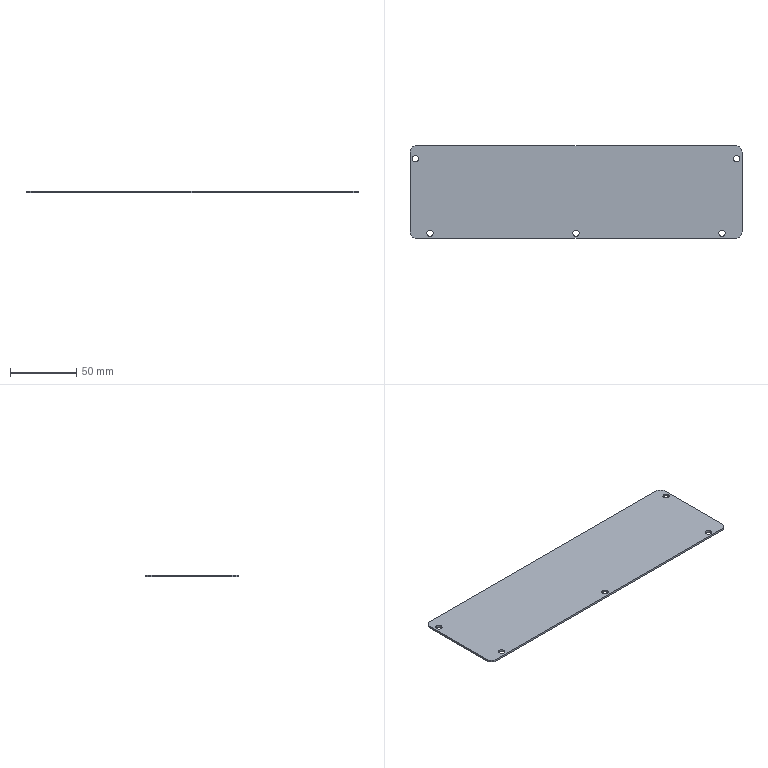Part | SolidWorks | features BreakCorner 1, FlatPattern 1, HoleWzd 1, SMBaseFlange 1, SheetMetal 1 | 1 solid | 20 faces | box 250 x 70 x 1.5 mm | volume 26082 mm3 | cylinder 14 | plane 6 | commonest cylinder face diameters 4.8 x10 10 x4
STEP:
#1=CARTESIAN_POINT('',(123.4,25.,0.));
#2=VERTEX_POINT('',#1);
#3=CARTESIAN_POINT('',(118.6,25.,0.));
#4=VERTEX_POINT('',#3);
#5=CARTESIAN_POINT('',(121.,25.,0.));
#6=DIRECTION('',(0.,0.,-1.));
#7=DIRECTION('',(-1.,0.,0.));
#8=AXIS2_PLACEMENT_3D('',#5,#6,#7);
#9=CIRCLE('',#8,2.4);
#10=EDGE_CURVE('',#2,#4,#9,.T.);
#11=ORIENTED_EDGE('',*,*,#10,.F.);
#12=CARTESIAN_POINT('',(123.4,25.,-1.5));
#13=VERTEX_POINT('',#12);
#14=CARTESIAN_POINT('',(123.4,25.,-1.5));
#15=DIRECTION('',(0.,0.,-1.));
#16=VECTOR('',#15,1000.);
#17=LINE('',#14,#16);
#18=EDGE_CURVE('',#2,#13,#17,.T.);
#19=ORIENTED_EDGE('',*,*,#18,.T.);
#20=CARTESIAN_POINT('',(118.6,25.,-1.5));
#21=VERTEX_POINT('',#20);
#22=CARTESIAN_POINT('',(121.,25.,-1.5));
#23=DIRECTION('',(0.,0.,-1.));
#24=DIRECTION('',(-1.,0.,0.));
#25=AXIS2_PLACEMENT_3D('',#22,#23,#24);
#26=CIRCLE('',#25,2.4);
#27=EDGE_CURVE('',#13,#21,#26,.T.);
#28=ORIENTED_EDGE('',*,*,#27,.T.);
#29=CARTESIAN_POINT('',(118.6,25.,-1.5));
#30=DIRECTION('',(0.,0.,-1.));
#31=VECTOR('',#30,1000.);
#32=LINE('',#29,#31);
#33=EDGE_CURVE('',#4,#21,#32,.T.);
#34=ORIENTED_EDGE('',*,*,#33,.F.);
#35=EDGE_LOOP('',(#11,#19,#28,#34));
#36=FACE_OUTER_BOUND('',#35,.T.);
#37=CARTESIAN_POINT('',(121.,25.,-1.5));
#38=DIRECTION('',(0.,0.,-1.));
#39=DIRECTION('',(-1.,0.,0.));
#40=AXIS2_PLACEMENT_3D('',#37,#38,#39);
#41=CYLINDRICAL_SURFACE('',#40,2.4);
#42=ADVANCED_FACE('',(#36),#41,.F.);
#43=CARTESIAN_POINT('',(112.4,-31.,0.));
#44=VERTEX_POINT('',#43);
#45=CARTESIAN_POINT('',(107.6,-31.,0.));
#46=VERTEX_POINT('',#45);
#47=CARTESIAN_POINT('',(110.,-31.,0.));
#48=DIRECTION('',(0.,0.,-1.));
#49=DIRECTION('',(-1.,0.,0.));
#50=AXIS2_PLACEMENT_3D('',#47,#48,#49);
#51=CIRCLE('',#50,2.4);
#52=EDGE_CURVE('',#44,#46,#51,.T.);
#53=ORIENTED_EDGE('',*,*,#52,.F.);
#54=CARTESIAN_POINT('',(112.4,-31.,-1.5));
#55=VERTEX_POINT('',#54);
#56=CARTESIAN_POINT('',(112.4,-31.,-1.5));
#57=DIRECTION('',(0.,0.,-1.));
#58=VECTOR('',#57,1000.);
#59=LINE('',#56,#58);
#60=EDGE_CURVE('',#44,#55,#59,.T.);
#61=ORIENTED_EDGE('',*,*,#60,.T.);
#62=CARTESIAN_POINT('',(107.6,-31.,-1.5));
#63=VERTEX_POINT('',#62);
#64=CARTESIAN_POINT('',(110.,-31.,-1.5));
#65=DIRECTION('',(0.,0.,-1.));
#66=DIRECTION('',(-1.,0.,0.));
#67=AXIS2_PLACEMENT_3D('',#64,#65,#66);
#68=CIRCLE('',#67,2.4);
#69=EDGE_CURVE('',#55,#63,#68,.T.);
#70=ORIENTED_EDGE('',*,*,#69,.T.);
#71=CARTESIAN_POINT('',(107.6,-31.,-1.5));
#72=DIRECTION('',(0.,0.,-1.));
#73=VECTOR('',#72,1000.);
#74=LINE('',#71,#73);
#75=EDGE_CURVE('',#46,#63,#74,.T.);
#76=ORIENTED_EDGE('',*,*,#75,.F.);
#77=EDGE_LOOP('',(#53,#61,#70,#76));
#78=FACE_OUTER_BOUND('',#77,.T.);
#79=CARTESIAN_POINT('',(110.,-31.,-1.5));
#80=DIRECTION('',(0.,0.,-1.));
#81=DIRECTION('',(-1.,0.,0.));
#82=AXIS2_PLACEMENT_3D('',#79,#80,#81);
#83=CYLINDRICAL_SURFACE('',#82,2.4);
#84=ADVANCED_FACE('',(#78),#83,.F.);
#85=CARTESIAN_POINT('',(2.4,-31.,0.));
#86=VERTEX_POINT('',#85);
#87=CARTESIAN_POINT('',(-2.4,-31.,0.));
#88=VERTEX_POINT('',#87);
#89=CARTESIAN_POINT('',(0.,-31.,0.));
#90=DIRECTION('',(0.,0.,-1.));
#91=DIRECTION('',(-1.,0.,0.));
#92=AXIS2_PLACEMENT_3D('',#89,#90,#91);
#93=CIRCLE('',#92,2.4);
#94=EDGE_CURVE('',#86,#88,#93,.T.);
#95=ORIENTED_EDGE('',*,*,#94,.F.);
#96=CARTESIAN_POINT('',(2.4,-31.,-1.5));
#97=VERTEX_POINT('',#96);
#98=CARTESIAN_POINT('',(2.4,-31.,-1.5));
#99=DIRECTION('',(0.,0.,-1.));
#100=VECTOR('',#99,1000.);
#101=LINE('',#98,#100);
#102=EDGE_CURVE('',#86,#97,#101,.T.);
#103=ORIENTED_EDGE('',*,*,#102,.T.);
#104=CARTESIAN_POINT('',(-2.4,-31.,-1.5));
#105=VERTEX_POINT('',#104);
#106=CARTESIAN_POINT('',(0.,-31.,-1.5));
#107=DIRECTION('',(0.,0.,-1.));
#108=DIRECTION('',(-1.,0.,0.));
#109=AXIS2_PLACEMENT_3D('',#106,#107,#108);
#110=CIRCLE('',#109,2.4);
#111=EDGE_CURVE('',#97,#105,#110,.T.);
#112=ORIENTED_EDGE('',*,*,#111,.T.);
#113=CARTESIAN_POINT('',(-2.4,-31.,-1.5));
#114=DIRECTION('',(0.,0.,-1.));
#115=VECTOR('',#114,1000.);
#116=LINE('',#113,#115);
#117=EDGE_CURVE('',#88,#105,#116,.T.);
#118=ORIENTED_EDGE('',*,*,#117,.F.);
#119=EDGE_LOOP('',(#95,#103,#112,#118));
#120=FACE_OUTER_BOUND('',#119,.T.);
#121=CARTESIAN_POINT('',(0.,-31.,-1.5));
#122=DIRECTION('',(0.,0.,-1.));
#123=DIRECTION('',(-1.,0.,0.));
#124=AXIS2_PLACEMENT_3D('',#121,#122,#123);
#125=CYLINDRICAL_SURFACE('',#124,2.4);
#126=ADVANCED_FACE('',(#120),#125,.F.);
#127=CARTESIAN_POINT('',(-107.6,-31.,0.));
#128=VERTEX_POINT('',#127);
#129=CARTESIAN_POINT('',(-112.4,-31.,0.));
#130=VERTEX_POINT('',#129);
#131=CARTESIAN_POINT('',(-110.,-31.,0.));
#132=DIRECTION('',(0.,0.,-1.));
#133=DIRECTION('',(-1.,0.,0.));
#134=AXIS2_PLACEMENT_3D('',#131,#132,#133);
#135=CIRCLE('',#134,2.4);
#136=EDGE_CURVE('',#128,#130,#135,.T.);
#137=ORIENTED_EDGE('',*,*,#136,.F.);
#138=CARTESIAN_POINT('',(-107.6,-31.,-1.5));
#139=VERTEX_POINT('',#138);
#140=CARTESIAN_POINT('',(-107.6,-31.,-1.5));
#141=DIRECTION('',(0.,0.,-1.));
#142=VECTOR('',#141,1000.);
#143=LINE('',#140,#142);
#144=EDGE_CURVE('',#128,#139,#143,.T.);
#145=ORIENTED_EDGE('',*,*,#144,.T.);
#146=CARTESIAN_POINT('',(-112.4,-31.,-1.5));
#147=VERTEX_POINT('',#146);
#148=CARTESIAN_POINT('',(-110.,-31.,-1.5));
#149=DIRECTION('',(0.,0.,-1.));
#150=DIRECTION('',(-1.,0.,0.));
#151=AXIS2_PLACEMENT_3D('',#148,#149,#150);
#152=CIRCLE('',#151,2.4);
#153=EDGE_CURVE('',#139,#147,#152,.T.);
#154=ORIENTED_EDGE('',*,*,#153,.T.);
#155=CARTESIAN_POINT('',(-112.4,-31.,-1.5));
#156=DIRECTION('',(0.,0.,-1.));
#157=VECTOR('',#156,1000.);
#158=LINE('',#155,#157);
#159=EDGE_CURVE('',#130,#147,#158,.T.);
#160=ORIENTED_EDGE('',*,*,#159,.F.);
#161=EDGE_LOOP('',(#137,#145,#154,#160));
#162=FACE_OUTER_BOUND('',#161,.T.);
#163=CARTESIAN_POINT('',(-110.,-31.,-1.5));
#164=DIRECTION('',(0.,0.,-1.));
#165=DIRECTION('',(-1.,0.,0.));
#166=AXIS2_PLACEMENT_3D('',#163,#164,#165);
#167=CYLINDRICAL_SURFACE('',#166,2.4);
#168=ADVANCED_FACE('',(#162),#167,.F.);
#169=CARTESIAN_POINT('',(-118.6,25.,0.));
#170=VERTEX_POINT('',#169);
#171=CARTESIAN_POINT('',(-123.4,25.,0.));
#172=VERTEX_POINT('',#171);
#173=CARTESIAN_POINT('',(-121.,25.,0.));
#174=DIRECTION('',(0.,0.,-1.));
#175=DIRECTION('',(-1.,0.,0.));
#176=AXIS2_PLACEMENT_3D('',#173,#174,#175);
#177=CIRCLE('',#176,2.4);
#178=EDGE_CURVE('',#170,#172,#177,.T.);
#179=ORIENTED_EDGE('',*,*,#178,.F.);
#180=CARTESIAN_POINT('',(-118.6,25.,-1.5));
#181=VERTEX_POINT('',#180);
#182=CARTESIAN_POINT('',(-118.6,25.,-1.5));
#183=DIRECTION('',(0.,0.,-1.));
#184=VECTOR('',#183,1000.);
#185=LINE('',#182,#184);
#186=EDGE_CURVE('',#170,#181,#185,.T.);
#187=ORIENTED_EDGE('',*,*,#186,.T.);
#188=CARTESIAN_POINT('',(-123.4,25.,-1.5));
#189=VERTEX_POINT('',#188);
#190=CARTESIAN_POINT('',(-121.,25.,-1.5));
#191=DIRECTION('',(0.,0.,-1.));
#192=DIRECTION('',(-1.,0.,0.));
#193=AXIS2_PLACEMENT_3D('',#190,#191,#192);
#194=CIRCLE('',#193,2.4);
#195=EDGE_CURVE('',#181,#189,#194,.T.);
#196=ORIENTED_EDGE('',*,*,#195,.T.);
#197=CARTESIAN_POINT('',(-123.4,25.,-1.5));
#198=DIRECTION('',(0.,0.,-1.));
#199=VECTOR('',#198,1000.);
#200=LINE('',#197,#199);
#201=EDGE_CURVE('',#172,#189,#200,.T.);
#202=ORIENTED_EDGE('',*,*,#201,.F.);
#203=EDGE_LOOP('',(#179,#187,#196,#202));
#204=FACE_OUTER_BOUND('',#203,.T.);
#205=CARTESIAN_POINT('',(-121.,25.,-1.5));
#206=DIRECTION('',(0.,0.,-1.));
#207=DIRECTION('',(-1.,0.,0.));
#208=AXIS2_PLACEMENT_3D('',#205,#206,#207);
#209=CYLINDRICAL_SURFACE('',#208,2.4);
#210=ADVANCED_FACE('',(#204),#209,.F.);
#211=CARTESIAN_POINT('',(125.,-30.,-1.5));
#212=VERTEX_POINT('',#211);
#213=CARTESIAN_POINT('',(125.,30.,-1.5));
#214=VERTEX_POINT('',#213);
#215=CARTESIAN_POINT('',(125.,-35.,-1.5));
#216=DIRECTION('',(0.,1.,0.));
#217=VECTOR('',#216,1000.);
#218=LINE('',#215,#217);
#219=EDGE_CURVE('',#212,#214,#218,.T.);
#220=ORIENTED_EDGE('',*,*,#219,.T.);
#221=CARTESIAN_POINT('',(125.,30.,0.));
#222=VERTEX_POINT('',#221);
#223=CARTESIAN_POINT('',(125.,30.,-1.5));
#224=DIRECTION('',(0.,0.,1.));
#225=VECTOR('',#224,1000.);
#226=LINE('',#223,#225);
#227=EDGE_CURVE('',#214,#222,#226,.T.);
#228=ORIENTED_EDGE('',*,*,#227,.T.);
#229=CARTESIAN_POINT('',(125.,-30.,0.));
#230=VERTEX_POINT('',#229);
#231=CARTESIAN_POINT('',(125.,-35.,0.));
#232=DIRECTION('',(0.,1.,0.));
#233=VECTOR('',#232,1000.);
#234=LINE('',#231,#233);
#235=EDGE_CURVE('',#230,#222,#234,.T.);
#236=ORIENTED_EDGE('',*,*,#235,.F.);
#237=CARTESIAN_POINT('',(125.,-30.,-1.5));
#238=DIRECTION('',(0.,0.,-1.));
#239=VECTOR('',#238,1000.);
#240=LINE('',#237,#239);
#241=EDGE_CURVE('',#230,#212,#240,.T.);
#242=ORIENTED_EDGE('',*,*,#241,.T.);
#243=EDGE_LOOP('',(#220,#228,#236,#242));
#244=FACE_OUTER_BOUND('',#243,.T.);
#245=CARTESIAN_POINT('',(125.,-35.,-1.5));
#246=DIRECTION('',(1.,0.,0.));
#247=DIRECTION('',(0.,0.,-1.));
#248=AXIS2_PLACEMENT_3D('',#245,#246,#247);
#249=PLANE('',#248);
#250=ADVANCED_FACE('',(#244),#249,.T.);
#251=CARTESIAN_POINT('',(-120.,-35.,0.));
#252=VERTEX_POINT('',#251);
#253=CARTESIAN_POINT('',(120.,-35.,0.));
#254=VERTEX_POINT('',#253);
#255=CARTESIAN_POINT('',(-125.,-35.,0.));
#256=DIRECTION('',(1.,0.,0.));
#257=VECTOR('',#256,1000.);
#258=LINE('',#255,#257);
#259=EDGE_CURVE('',#252,#254,#258,.T.);
#260=ORIENTED_EDGE('',*,*,#259,.F.);
#261=CARTESIAN_POINT('',(-120.,-35.,-1.5));
#262=VERTEX_POINT('',#261);
#263=CARTESIAN_POINT('',(-120.,-35.,-1.5));
#264=DIRECTION('',(0.,0.,-1.));
#265=VECTOR('',#264,1000.);
#266=LINE('',#263,#265);
#267=EDGE_CURVE('',#252,#262,#266,.T.);
#268=ORIENTED_EDGE('',*,*,#267,.T.);
#269=CARTESIAN_POINT('',(120.,-35.,-1.5));
#270=VERTEX_POINT('',#269);
#271=CARTESIAN_POINT('',(-125.,-35.,-1.5));
#272=DIRECTION('',(1.,0.,0.));
#273=VECTOR('',#272,1000.);
#274=LINE('',#271,#273);
#275=EDGE_CURVE('',#262,#270,#274,.T.);
#276=ORIENTED_EDGE('',*,*,#275,.T.);
#277=CARTESIAN_POINT('',(120.,-35.,-1.5));
#278=DIRECTION('',(0.,0.,1.));
#279=VECTOR('',#278,1000.);
#280=LINE('',#277,#279);
#281=EDGE_CURVE('',#270,#254,#280,.T.);
#282=ORIENTED_EDGE('',*,*,#281,.T.);
#283=EDGE_LOOP('',(#260,#268,#276,#282));
#284=FACE_OUTER_BOUND('',#283,.T.);
#285=CARTESIAN_POINT('',(-125.,-35.,-1.5));
#286=DIRECTION('',(0.,-1.,0.));
#287=DIRECTION('',(0.,0.,-1.));
#288=AXIS2_PLACEMENT_3D('',#285,#286,#287);
#289=PLANE('',#288);
#290=ADVANCED_FACE('',(#284),#289,.T.);
#291=CARTESIAN_POINT('',(-125.,30.,0.));
#292=VERTEX_POINT('',#291);
#293=CARTESIAN_POINT('',(-125.,-30.,0.));
#294=VERTEX_POINT('',#293);
#295=CARTESIAN_POINT('',(-125.,-35.,0.));
#296=DIRECTION('',(0.,-1.,0.));
#297=VECTOR('',#296,1000.);
#298=LINE('',#295,#297);
#299=EDGE_CURVE('',#292,#294,#298,.T.);
#300=ORIENTED_EDGE('',*,*,#299,.F.);
#301=CARTESIAN_POINT('',(-125.,30.,-1.5));
#302=VERTEX_POINT('',#301);
#303=CARTESIAN_POINT('',(-125.,30.,-1.5));
#304=DIRECTION('',(0.,0.,-1.));
#305=VECTOR('',#304,1000.);
#306=LINE('',#303,#305);
#307=EDGE_CURVE('',#292,#302,#306,.T.);
#308=ORIENTED_EDGE('',*,*,#307,.T.);
#309=CARTESIAN_POINT('',(-125.,-30.,-1.5));
#310=VERTEX_POINT('',#309);
#311=CARTESIAN_POINT('',(-125.,-35.,-1.5));
#312=DIRECTION('',(0.,-1.,0.));
#313=VECTOR('',#312,1000.);
#314=LINE('',#311,#313);
#315=EDGE_CURVE('',#302,#310,#314,.T.);
#316=ORIENTED_EDGE('',*,*,#315,.T.);
#317=CARTESIAN_POINT('',(-125.,-30.,-1.5));
#318=DIRECTION('',(0.,0.,1.));
#319=VECTOR('',#318,1000.);
#320=LINE('',#317,#319);
#321=EDGE_CURVE('',#310,#294,#320,.T.);
#322=ORIENTED_EDGE('',*,*,#321,.T.);
#323=EDGE_LOOP('',(#300,#308,#316,#322));
#324=FACE_OUTER_BOUND('',#323,.T.);
#325=CARTESIAN_POINT('',(-125.,-35.,-1.5));
#326=DIRECTION('',(-1.,0.,0.));
#327=DIRECTION('',(0.,0.,1.));
#328=AXIS2_PLACEMENT_3D('',#325,#326,#327);
#329=PLANE('',#328);
#330=ADVANCED_FACE('',(#324),#329,.T.);
#331=CARTESIAN_POINT('',(120.,35.,0.));
#332=VERTEX_POINT('',#331);
#333=CARTESIAN_POINT('',(-120.,35.,0.));
#334=VERTEX_POINT('',#333);
#335=CARTESIAN_POINT('',(-125.,35.,0.));
#336=DIRECTION('',(-1.,0.,0.));
#337=VECTOR('',#336,1000.);
#338=LINE('',#335,#337);
#339=EDGE_CURVE('',#332,#334,#338,.T.);
#340=ORIENTED_EDGE('',*,*,#339,.F.);
#341=CARTESIAN_POINT('',(120.,35.,-1.5));
#342=VERTEX_POINT('',#341);
#343=CARTESIAN_POINT('',(120.,35.,-1.5));
#344=DIRECTION('',(0.,0.,-1.));
#345=VECTOR('',#344,1000.);
#346=LINE('',#343,#345);
#347=EDGE_CURVE('',#332,#342,#346,.T.);
#348=ORIENTED_EDGE('',*,*,#347,.T.);
#349=CARTESIAN_POINT('',(-120.,35.,-1.5));
#350=VERTEX_POINT('',#349);
#351=CARTESIAN_POINT('',(-125.,35.,-1.5));
#352=DIRECTION('',(-1.,0.,0.));
#353=VECTOR('',#352,1000.);
#354=LINE('',#351,#353);
#355=EDGE_CURVE('',#342,#350,#354,.T.);
#356=ORIENTED_EDGE('',*,*,#355,.T.);
#357=CARTESIAN_POINT('',(-120.,35.,-1.5));
#358=DIRECTION('',(0.,0.,1.));
#359=VECTOR('',#358,1000.);
#360=LINE('',#357,#359);
#361=EDGE_CURVE('',#350,#334,#360,.T.);
#362=ORIENTED_EDGE('',*,*,#361,.T.);
#363=EDGE_LOOP('',(#340,#348,#356,#362));
#364=FACE_OUTER_BOUND('',#363,.T.);
#365=CARTESIAN_POINT('',(-125.,35.,-1.5));
#366=DIRECTION('',(0.,1.,0.));
#367=DIRECTION('',(0.,0.,1.));
#368=AXIS2_PLACEMENT_3D('',#365,#366,#367);
#369=PLANE('',#368);
#370=ADVANCED_FACE('',(#364),#369,.T.);
#371=CARTESIAN_POINT('',(121.,25.,-1.5));
#372=DIRECTION('',(0.,0.,-1.));
#373=DIRECTION('',(-1.,0.,0.));
#374=AXIS2_PLACEMENT_3D('',#371,#372,#373);
#375=CIRCLE('',#374,2.4);
#376=EDGE_CURVE('',#21,#13,#375,.T.);
#377=ORIENTED_EDGE('',*,*,#376,.F.);
#378=ORIENTED_EDGE('',*,*,#27,.F.);
#379=EDGE_LOOP('',(#377,#378));
#380=FACE_BOUND('',#379,.T.);
#381=CARTESIAN_POINT('',(110.,-31.,-1.5));
#382=DIRECTION('',(0.,0.,-1.));
#383=DIRECTION('',(-1.,0.,0.));
#384=AXIS2_PLACEMENT_3D('',#381,#382,#383);
#385=CIRCLE('',#384,2.4);
#386=EDGE_CURVE('',#63,#55,#385,.T.);
#387=ORIENTED_EDGE('',*,*,#386,.F.);
#388=ORIENTED_EDGE('',*,*,#69,.F.);
#389=EDGE_LOOP('',(#387,#388));
#390=FACE_BOUND('',#389,.T.);
#391=CARTESIAN_POINT('',(0.,-31.,-1.5));
#392=DIRECTION('',(0.,0.,-1.));
#393=DIRECTION('',(-1.,0.,0.));
#394=AXIS2_PLACEMENT_3D('',#391,#392,#393);
#395=CIRCLE('',#394,2.4);
#396=EDGE_CURVE('',#105,#97,#395,.T.);
#397=ORIENTED_EDGE('',*,*,#396,.F.);
#398=ORIENTED_EDGE('',*,*,#111,.F.);
#399=EDGE_LOOP('',(#397,#398));
#400=FACE_BOUND('',#399,.T.);
#401=CARTESIAN_POINT('',(-110.,-31.,-1.5));
#402=DIRECTION('',(0.,0.,-1.));
#403=DIRECTION('',(-1.,0.,0.));
#404=AXIS2_PLACEMENT_3D('',#401,#402,#403);
#405=CIRCLE('',#404,2.4);
#406=EDGE_CURVE('',#147,#139,#405,.T.);
#407=ORIENTED_EDGE('',*,*,#406,.F.);
#408=ORIENTED_EDGE('',*,*,#153,.F.);
#409=EDGE_LOOP('',(#407,#408));
#410=FACE_BOUND('',#409,.T.);
#411=CARTESIAN_POINT('',(-121.,25.,-1.5));
#412=DIRECTION('',(0.,0.,-1.));
#413=DIRECTION('',(-1.,0.,0.));
#414=AXIS2_PLACEMENT_3D('',#411,#412,#413);
#415=CIRCLE('',#414,2.4);
#416=EDGE_CURVE('',#189,#181,#415,.T.);
#417=ORIENTED_EDGE('',*,*,#416,.F.);
#418=ORIENTED_EDGE('',*,*,#195,.F.);
#419=EDGE_LOOP('',(#417,#418));
#420=FACE_BOUND('',#419,.T.);
#421=ORIENTED_EDGE('',*,*,#355,.F.);
#422=CARTESIAN_POINT('',(120.,30.,-1.5));
#423=DIRECTION('',(0.,0.,-1.));
#424=DIRECTION('',(-1.,0.,0.));
#425=AXIS2_PLACEMENT_3D('',#422,#423,#424);
#426=CIRCLE('',#425,5.);
#427=EDGE_CURVE('',#342,#214,#426,.T.);
#428=ORIENTED_EDGE('',*,*,#427,.T.);
#429=ORIENTED_EDGE('',*,*,#219,.F.);
#430=CARTESIAN_POINT('',(120.,-30.,-1.5));
#431=DIRECTION('',(0.,0.,-1.));
#432=DIRECTION('',(-1.,0.,0.));
#433=AXIS2_PLACEMENT_3D('',#430,#431,#432);
#434=CIRCLE('',#433,5.);
#435=EDGE_CURVE('',#212,#270,#434,.T.);
#436=ORIENTED_EDGE('',*,*,#435,.T.);
#437=ORIENTED_EDGE('',*,*,#275,.F.);
#438=CARTESIAN_POINT('',(-120.,-30.,-1.5));
#439=DIRECTION('',(0.,0.,-1.));
#440=DIRECTION('',(-1.,0.,0.));
#441=AXIS2_PLACEMENT_3D('',#438,#439,#440);
#442=CIRCLE('',#441,5.);
#443=EDGE_CURVE('',#262,#310,#442,.T.);
#444=ORIENTED_EDGE('',*,*,#443,.T.);
#445=ORIENTED_EDGE('',*,*,#315,.F.);
#446=CARTESIAN_POINT('',(-120.,30.,-1.5));
#447=DIRECTION('',(0.,0.,-1.));
#448=DIRECTION('',(-1.,0.,0.));
#449=AXIS2_PLACEMENT_3D('',#446,#447,#448);
#450=CIRCLE('',#449,5.);
#451=EDGE_CURVE('',#302,#350,#450,.T.);
#452=ORIENTED_EDGE('',*,*,#451,.T.);
#453=EDGE_LOOP('',(#421,#428,#429,#436,#437,#444,#445,#452));
#454=FACE_OUTER_BOUND('',#453,.T.);
#455=CARTESIAN_POINT('',(0.,0.,-1.5));
#456=DIRECTION('',(0.,0.,-1.));
#457=DIRECTION('',(-1.,0.,0.));
#458=AXIS2_PLACEMENT_3D('',#455,#456,#457);
#459=PLANE('',#458);
#460=ADVANCED_FACE('',(#380,#390,#400,#410,#420,#454),#459,.T.);
#461=CARTESIAN_POINT('',(121.,25.,0.));
#462=DIRECTION('',(0.,0.,-1.));
#463=DIRECTION('',(-1.,0.,0.));
#464=AXIS2_PLACEMENT_3D('',#461,#462,#463);
#465=CIRCLE('',#464,2.4);
#466=EDGE_CURVE('',#4,#2,#465,.T.);
#467=ORIENTED_EDGE('',*,*,#466,.T.);
#468=ORIENTED_EDGE('',*,*,#10,.T.);
#469=EDGE_LOOP('',(#467,#468));
#470=FACE_BOUND('',#469,.T.);
#471=CARTESIAN_POINT('',(110.,-31.,0.));
#472=DIRECTION('',(0.,0.,-1.));
#473=DIRECTION('',(-1.,0.,0.));
#474=AXIS2_PLACEMENT_3D('',#471,#472,#473);
#475=CIRCLE('',#474,2.4);
#476=EDGE_CURVE('',#46,#44,#475,.T.);
#477=ORIENTED_EDGE('',*,*,#476,.T.);
#478=ORIENTED_EDGE('',*,*,#52,.T.);
#479=EDGE_LOOP('',(#477,#478));
#480=FACE_BOUND('',#479,.T.);
#481=CARTESIAN_POINT('',(0.,-31.,0.));
#482=DIRECTION('',(0.,0.,-1.));
#483=DIRECTION('',(-1.,0.,0.));
#484=AXIS2_PLACEMENT_3D('',#481,#482,#483);
#485=CIRCLE('',#484,2.4);
#486=EDGE_CURVE('',#88,#86,#485,.T.);
#487=ORIENTED_EDGE('',*,*,#486,.T.);
#488=ORIENTED_EDGE('',*,*,#94,.T.);
#489=EDGE_LOOP('',(#487,#488));
#490=FACE_BOUND('',#489,.T.);
#491=CARTESIAN_POINT('',(-110.,-31.,0.));
#492=DIRECTION('',(0.,0.,-1.));
#493=DIRECTION('',(-1.,0.,0.));
#494=AXIS2_PLACEMENT_3D('',#491,#492,#493);
#495=CIRCLE('',#494,2.4);
#496=EDGE_CURVE('',#130,#128,#495,.T.);
#497=ORIENTED_EDGE('',*,*,#496,.T.);
#498=ORIENTED_EDGE('',*,*,#136,.T.);
#499=EDGE_LOOP('',(#497,#498));
#500=FACE_BOUND('',#499,.T.);
#501=CARTESIAN_POINT('',(-121.,25.,0.));
#502=DIRECTION('',(0.,0.,-1.));
#503=DIRECTION('',(-1.,0.,0.));
#504=AXIS2_PLACEMENT_3D('',#501,#502,#503);
#505=CIRCLE('',#504,2.4);
#506=EDGE_CURVE('',#172,#170,#505,.T.);
#507=ORIENTED_EDGE('',*,*,#506,.T.);
#508=ORIENTED_EDGE('',*,*,#178,.T.);
#509=EDGE_LOOP('',(#507,#508));
#510=FACE_BOUND('',#509,.T.);
#511=ORIENTED_EDGE('',*,*,#235,.T.);
#512=CARTESIAN_POINT('',(120.,30.,0.));
#513=DIRECTION('',(0.,0.,1.));
#514=DIRECTION('',(-1.,0.,0.));
#515=AXIS2_PLACEMENT_3D('',#512,#513,#514);
#516=CIRCLE('',#515,5.);
#517=EDGE_CURVE('',#222,#332,#516,.T.);
#518=ORIENTED_EDGE('',*,*,#517,.T.);
#519=ORIENTED_EDGE('',*,*,#339,.T.);
#520=CARTESIAN_POINT('',(-120.,30.,0.));
#521=DIRECTION('',(0.,0.,1.));
#522=DIRECTION('',(-1.,0.,0.));
#523=AXIS2_PLACEMENT_3D('',#520,#521,#522);
#524=CIRCLE('',#523,5.);
#525=EDGE_CURVE('',#334,#292,#524,.T.);
#526=ORIENTED_EDGE('',*,*,#525,.T.);
#527=ORIENTED_EDGE('',*,*,#299,.T.);
#528=CARTESIAN_POINT('',(-120.,-30.,0.));
#529=DIRECTION('',(0.,0.,1.));
#530=DIRECTION('',(-1.,0.,0.));
#531=AXIS2_PLACEMENT_3D('',#528,#529,#530);
#532=CIRCLE('',#531,5.);
#533=EDGE_CURVE('',#294,#252,#532,.T.);
#534=ORIENTED_EDGE('',*,*,#533,.T.);
#535=ORIENTED_EDGE('',*,*,#259,.T.);
#536=CARTESIAN_POINT('',(120.,-30.,0.));
#537=DIRECTION('',(0.,0.,1.));
#538=DIRECTION('',(-1.,0.,0.));
#539=AXIS2_PLACEMENT_3D('',#536,#537,#538);
#540=CIRCLE('',#539,5.);
#541=EDGE_CURVE('',#254,#230,#540,.T.);
#542=ORIENTED_EDGE('',*,*,#541,.T.);
#543=EDGE_LOOP('',(#511,#518,#519,#526,#527,#534,#535,#542));
#544=FACE_OUTER_BOUND('',#543,.T.);
#545=CARTESIAN_POINT('',(0.,0.,0.));
#546=DIRECTION('',(0.,0.,-1.));
#547=DIRECTION('',(-1.,0.,0.));
#548=AXIS2_PLACEMENT_3D('',#545,#546,#547);
#549=PLANE('',#548);
#550=ADVANCED_FACE('',(#470,#480,#490,#500,#510,#544),#549,.F.);
#551=ORIENTED_EDGE('',*,*,#186,.F.);
#552=ORIENTED_EDGE('',*,*,#506,.F.);
#553=ORIENTED_EDGE('',*,*,#201,.T.);
#554=ORIENTED_EDGE('',*,*,#416,.T.);
#555=EDGE_LOOP('',(#551,#552,#553,#554));
#556=FACE_OUTER_BOUND('',#555,.T.);
#557=CARTESIAN_POINT('',(-121.,25.,-1.5));
#558=DIRECTION('',(0.,0.,-1.));
#559=DIRECTION('',(-1.,0.,0.));
#560=AXIS2_PLACEMENT_3D('',#557,#558,#559);
#561=CYLINDRICAL_SURFACE('',#560,2.4);
#562=ADVANCED_FACE('',(#556),#561,.F.);
#563=ORIENTED_EDGE('',*,*,#144,.F.);
#564=ORIENTED_EDGE('',*,*,#496,.F.);
#565=ORIENTED_EDGE('',*,*,#159,.T.);
#566=ORIENTED_EDGE('',*,*,#406,.T.);
#567=EDGE_LOOP('',(#563,#564,#565,#566));
#568=FACE_OUTER_BOUND('',#567,.T.);
#569=CARTESIAN_POINT('',(-110.,-31.,-1.5));
#570=DIRECTION('',(0.,0.,-1.));
#571=DIRECTION('',(-1.,0.,0.));
#572=AXIS2_PLACEMENT_3D('',#569,#570,#571);
#573=CYLINDRICAL_SURFACE('',#572,2.4);
#574=ADVANCED_FACE('',(#568),#573,.F.);
#575=ORIENTED_EDGE('',*,*,#102,.F.);
#576=ORIENTED_EDGE('',*,*,#486,.F.);
#577=ORIENTED_EDGE('',*,*,#117,.T.);
#578=ORIENTED_EDGE('',*,*,#396,.T.);
#579=EDGE_LOOP('',(#575,#576,#577,#578));
#580=FACE_OUTER_BOUND('',#579,.T.);
#581=CARTESIAN_POINT('',(0.,-31.,-1.5));
#582=DIRECTION('',(0.,0.,-1.));
#583=DIRECTION('',(-1.,0.,0.));
#584=AXIS2_PLACEMENT_3D('',#581,#582,#583);
#585=CYLINDRICAL_SURFACE('',#584,2.4);
#586=ADVANCED_FACE('',(#580),#585,.F.);
#587=ORIENTED_EDGE('',*,*,#60,.F.);
#588=ORIENTED_EDGE('',*,*,#476,.F.);
#589=ORIENTED_EDGE('',*,*,#75,.T.);
#590=ORIENTED_EDGE('',*,*,#386,.T.);
#591=EDGE_LOOP('',(#587,#588,#589,#590));
#592=FACE_OUTER_BOUND('',#591,.T.);
#593=CARTESIAN_POINT('',(110.,-31.,-1.5));
#594=DIRECTION('',(0.,0.,-1.));
#595=DIRECTION('',(-1.,0.,0.));
#596=AXIS2_PLACEMENT_3D('',#593,#594,#595);
#597=CYLINDRICAL_SURFACE('',#596,2.4);
#598=ADVANCED_FACE('',(#592),#597,.F.);
#599=ORIENTED_EDGE('',*,*,#18,.F.);
#600=ORIENTED_EDGE('',*,*,#466,.F.);
#601=ORIENTED_EDGE('',*,*,#33,.T.);
#602=ORIENTED_EDGE('',*,*,#376,.T.);
#603=EDGE_LOOP('',(#599,#600,#601,#602));
#604=FACE_OUTER_BOUND('',#603,.T.);
#605=CARTESIAN_POINT('',(121.,25.,-1.5));
#606=DIRECTION('',(0.,0.,-1.));
#607=DIRECTION('',(-1.,0.,0.));
#608=AXIS2_PLACEMENT_3D('',#605,#606,#607);
#609=CYLINDRICAL_SURFACE('',#608,2.4);
#610=ADVANCED_FACE('',(#604),#609,.F.);
#611=ORIENTED_EDGE('',*,*,#427,.F.);
#612=ORIENTED_EDGE('',*,*,#347,.F.);
#613=ORIENTED_EDGE('',*,*,#517,.F.);
#614=ORIENTED_EDGE('',*,*,#227,.F.);
#615=EDGE_LOOP('',(#611,#612,#613,#614));
#616=FACE_OUTER_BOUND('',#615,.T.);
#617=CARTESIAN_POINT('',(120.,30.,-1.5));
#618=DIRECTION('',(0.,0.,1.));
#619=DIRECTION('',(1.,0.,0.));
#620=AXIS2_PLACEMENT_3D('',#617,#618,#619);
#621=CYLINDRICAL_SURFACE('',#620,5.);
#622=ADVANCED_FACE('',(#616),#621,.T.);
#623=ORIENTED_EDGE('',*,*,#451,.F.);
#624=ORIENTED_EDGE('',*,*,#307,.F.);
#625=ORIENTED_EDGE('',*,*,#525,.F.);
#626=ORIENTED_EDGE('',*,*,#361,.F.);
#627=EDGE_LOOP('',(#623,#624,#625,#626));
#628=FACE_OUTER_BOUND('',#627,.T.);
#629=CARTESIAN_POINT('',(-120.,30.,-1.5));
#630=DIRECTION('',(0.,0.,1.));
#631=DIRECTION('',(1.,0.,0.));
#632=AXIS2_PLACEMENT_3D('',#629,#630,#631);
#633=CYLINDRICAL_SURFACE('',#632,5.);
#634=ADVANCED_FACE('',(#628),#633,.T.);
#635=ORIENTED_EDGE('',*,*,#443,.F.);
#636=ORIENTED_EDGE('',*,*,#267,.F.);
#637=ORIENTED_EDGE('',*,*,#533,.F.);
#638=ORIENTED_EDGE('',*,*,#321,.F.);
#639=EDGE_LOOP('',(#635,#636,#637,#638));
#640=FACE_OUTER_BOUND('',#639,.T.);
#641=CARTESIAN_POINT('',(-120.,-30.,-1.5));
#642=DIRECTION('',(0.,0.,1.));
#643=DIRECTION('',(1.,0.,0.));
#644=AXIS2_PLACEMENT_3D('',#641,#642,#643);
#645=CYLINDRICAL_SURFACE('',#644,5.);
#646=ADVANCED_FACE('',(#640),#645,.T.);
#647=ORIENTED_EDGE('',*,*,#435,.F.);
#648=ORIENTED_EDGE('',*,*,#241,.F.);
#649=ORIENTED_EDGE('',*,*,#541,.F.);
#650=ORIENTED_EDGE('',*,*,#281,.F.);
#651=EDGE_LOOP('',(#647,#648,#649,#650));
#652=FACE_OUTER_BOUND('',#651,.T.);
#653=CARTESIAN_POINT('',(120.,-30.,-1.5));
#654=DIRECTION('',(0.,0.,1.));
#655=DIRECTION('',(1.,0.,0.));
#656=AXIS2_PLACEMENT_3D('',#653,#654,#655);
#657=CYLINDRICAL_SURFACE('',#656,5.);
#658=ADVANCED_FACE('',(#652),#657,.T.);
#659=CLOSED_SHELL('',(#42,#84,#126,#168,#210,#250,#290,#330,#370,#460,#550,#562,#574,#586,#598,#610,#622,#634,#646,#658));
#660=MANIFOLD_SOLID_BREP('',#659);
#661=CARTESIAN_POINT('',(0.,0.,0.));
#662=DIRECTION('',(0.,0.,1.));
#663=DIRECTION('',(1.,0.,0.));
#664=AXIS2_PLACEMENT_3D('',#661,#662,#663);
#665=(LENGTH_UNIT()NAMED_UNIT(*)SI_UNIT(.MILLI.,.METRE.));
#666=UNCERTAINTY_MEASURE_WITH_UNIT(LENGTH_MEASURE(0.00001),#665,'','');
#667=(NAMED_UNIT(*)PLANE_ANGLE_UNIT()SI_UNIT($,.RADIAN.));
#668=(NAMED_UNIT(*)SI_UNIT($,.STERADIAN.)SOLID_ANGLE_UNIT());
#669=(GEOMETRIC_REPRESENTATION_CONTEXT(3)GLOBAL_UNCERTAINTY_ASSIGNED_CONTEXT((#666))GLOBAL_UNIT_ASSIGNED_CONTEXT((#665,#667,#668))REPRESENTATION_CONTEXT('',''));
#670=ADVANCED_BREP_SHAPE_REPRESENTATION('',(#660,#664),#669);